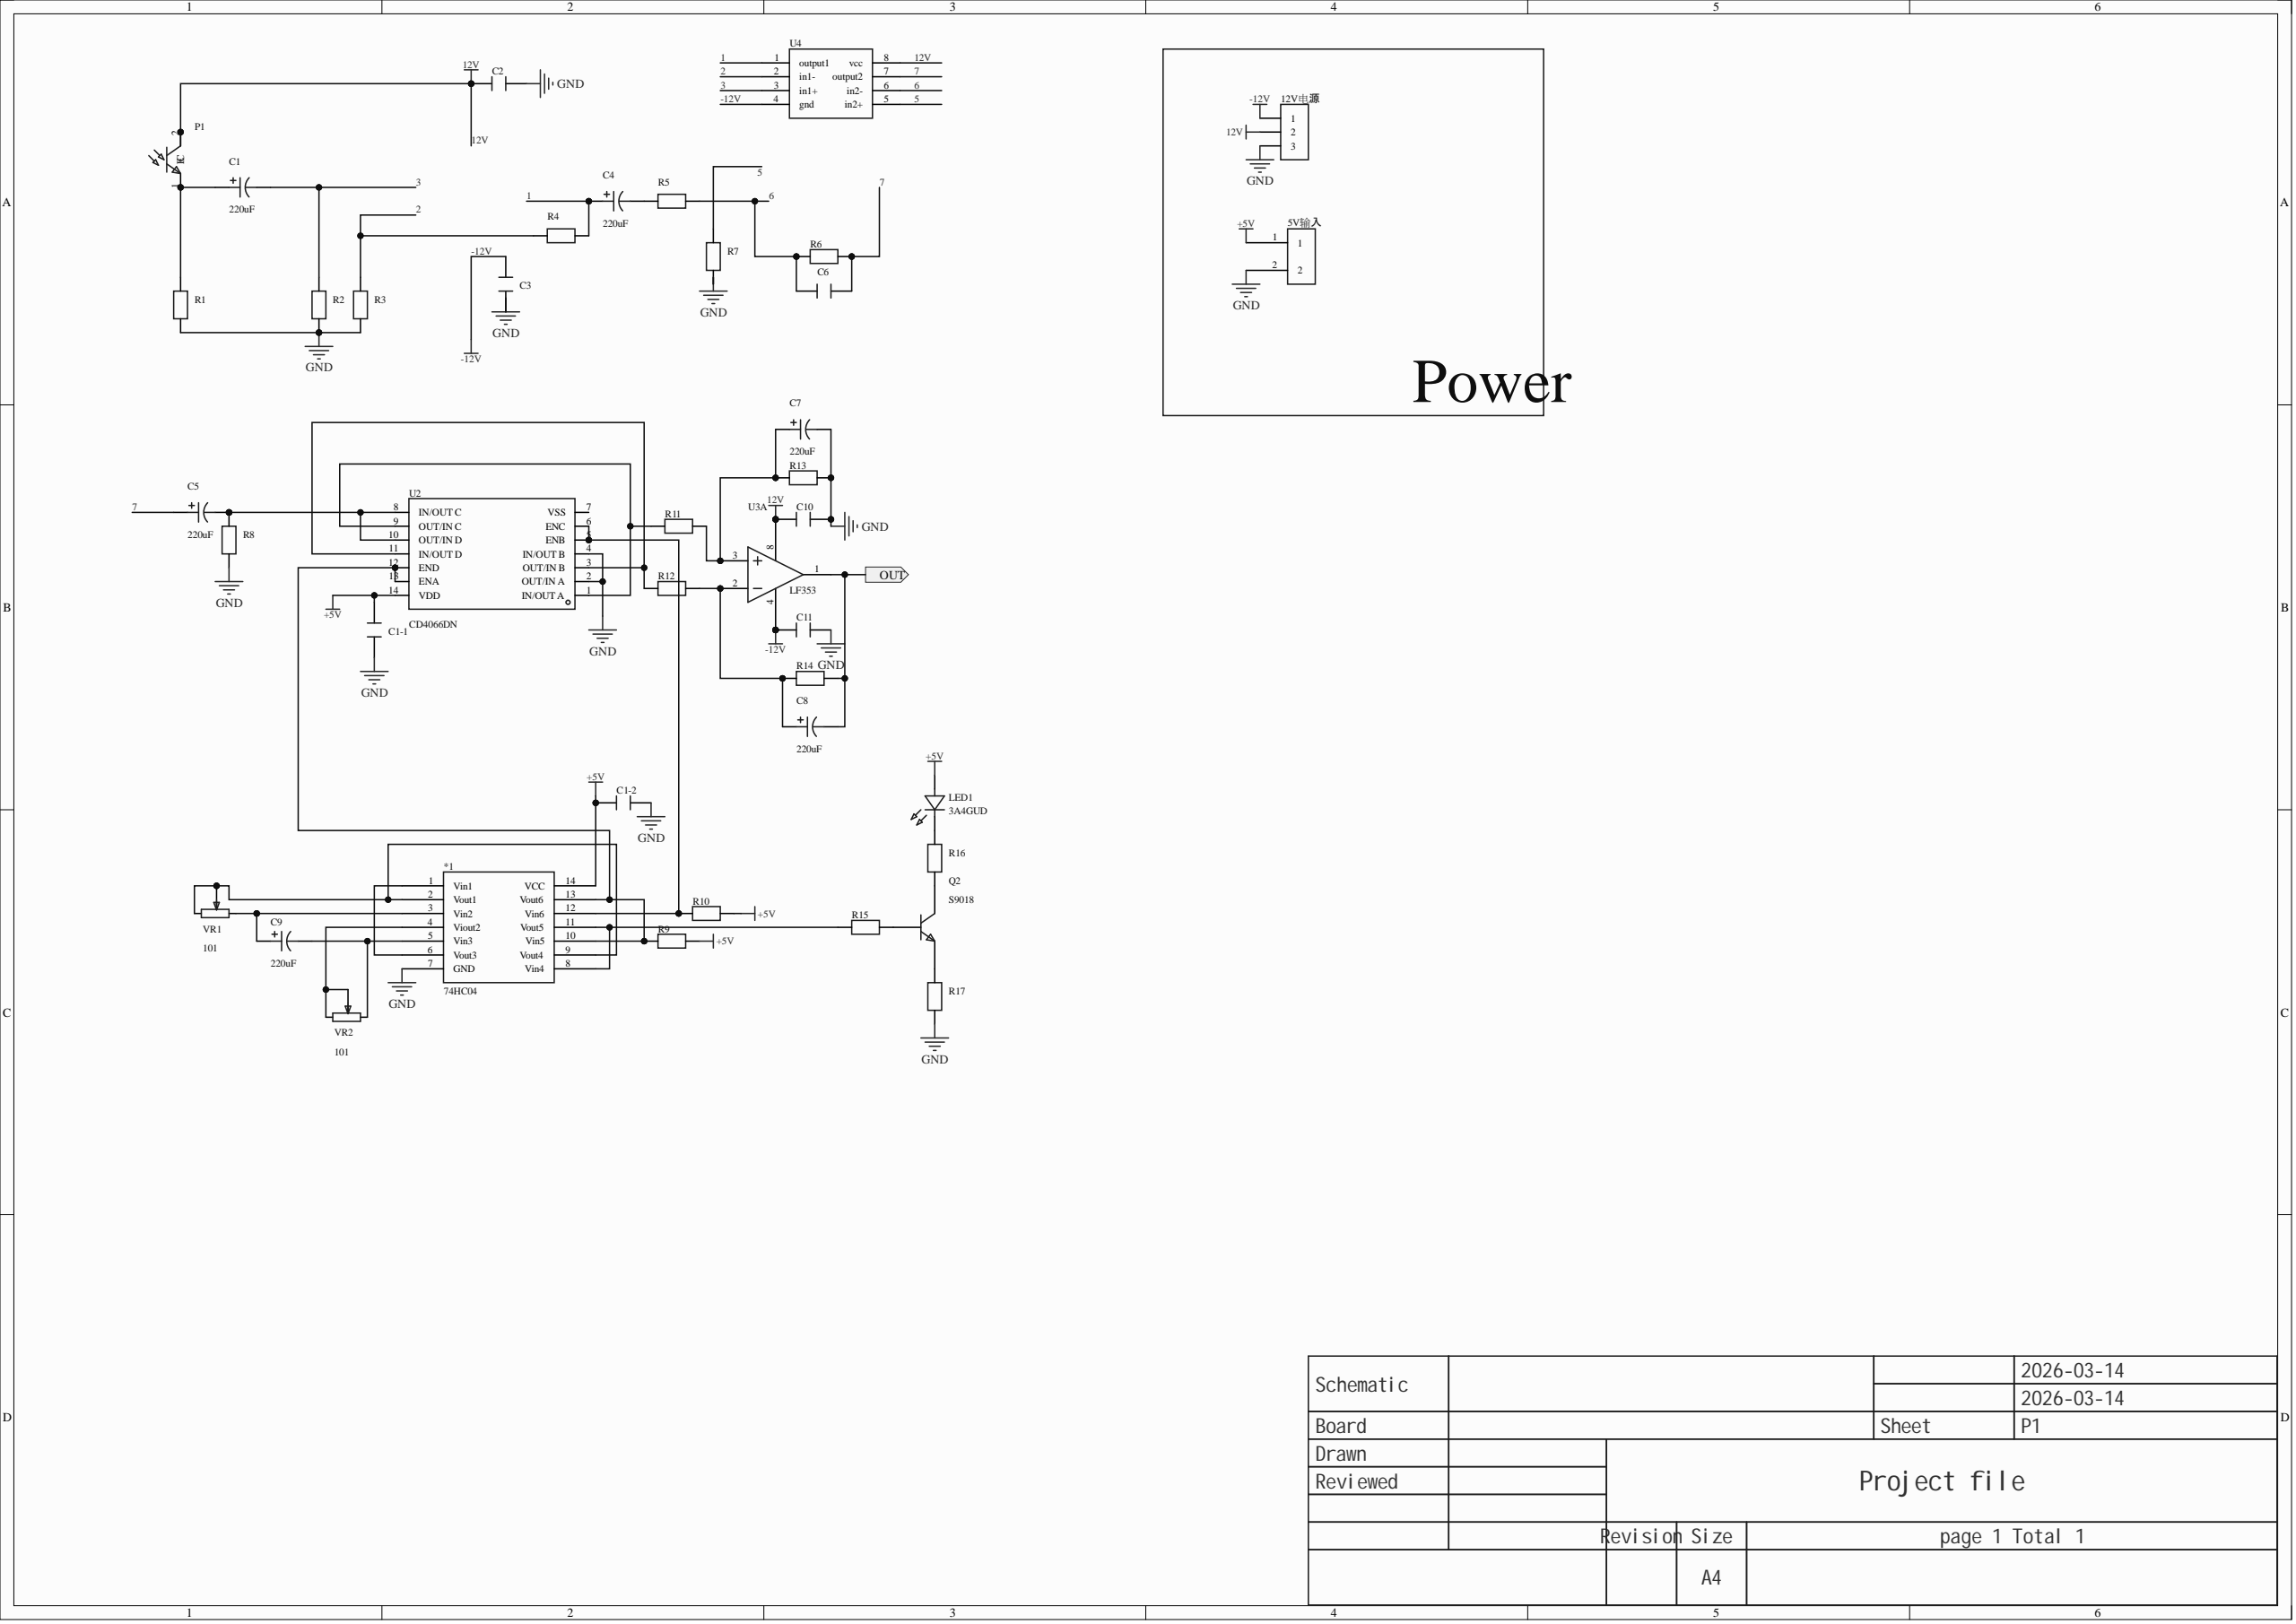Circuit board | Altium Designer | 41 parts | 30 nets
Bill of materials:
Comment,Description,Designator,Footprint,LibRef,Quantity
"74HC04","","*1","DIP14","74HC04","1"
"5V output","","5V输入","2INT","2PIN","1"
"3PIN","","12V电源","3PIN","3PIN","1"
"","","C1-1, C1-2, C2, C3, C6, C10, C11","电容直插","电容直插","7"
"220uF","Capacitance:220uF;Tolerance:±20%;Rated voltage:16V;Ripple current:300mA@100kHz;Equivalent series resistance(ESR):220mO@100kHz;","C1, C4, C5, C7, C8, C9","CAP-TH_BD6.3-P2.50-D0.5-FD","ERG16V220M6X7","6"
"3A4GUD","Lamp holder type:3mm round lamp holder;Illumination color:Emerald green;Forward voltage(Vf):2.8V~3.2V;Forward current:20mA;Wavelength:520nm~525nm;Lens color:Green lens;Color temperature:-;Luminous intensity:8000mcd~12000mcd;Viewing angle:30°;Operating temperature:-40℃~+85℃;","LED1","LED-TH_BD3.5-P2.54-RD-GREEN","3A4GUD","1"
"","","P1","LED_D3.0mm_Horizontal_O1.27mm_Z2.0mm","LED-3MM-红外接收","1"
"S9018","Transistor type:NPN;Collector-emitter breakdown voltage(Vceo):18V;Collector current(Ic):50mA;Power(Pd):400mW;Collector cutoff current(Icbo):100nA;Collector-emitter saturation voltage(VCE(sat)@Ic,Ib):500mV@10mA,1mA;DC current gain(hFE@Ic,Vce):97@1mA,5V;Transition frequency(fT):800MHz;Operating temperature:+150℃@(Tj);","Q2","TO-92-3_L4.9-W3.7-P1.27-L","S9018","1"
"","Through-hole resistor","R1, R2, R3, R4, R5, R6, R7, R8, R9, R10, R11, R12, R13, R14, R15, R16, R17","D45-V(直插)","直插电阻","17"
"CD4066DN","Switch circuit:1:1;Channels:4;On-resistance(Ron):125O;","U2","PDIP-14_L19.3-W6.5-P2.54-LS7.6-BL","CD4066DN","1"
"LF353","","U3","DIP-8","LF353","1"
"","","U4","DIP-8_L9.9-W6.4-P2.54-LS7.6-BL","lf353","1"
"101","","VR1, VR2","3296W","3296","2"
Netlist (Protel format):
[
5V输入
2INT
5V output



]
[
12V电源
3PIN
3PIN



]
[
*1
DIP14
74HC04



]
[
C1
CAP-TH_BD6.3-P2.50-D0.5-FD
220uF



]
[
C1-1
电容直插




]
[
C1-2
电容直插




]
[
C2
电容直插




]
[
C3
电容直插




]
[
C4
CAP-TH_BD6.3-P2.50-D0.5-FD
220uF



]
[
C5
CAP-TH_BD6.3-P2.50-D0.5-FD
220uF



]
[
C6
电容直插




]
[
C7
CAP-TH_BD6.3-P2.50-D0.5-FD
220uF



]
[
C8
CAP-TH_BD6.3-P2.50-D0.5-FD
220uF



]
[
C9
CAP-TH_BD6.3-P2.50-D0.5-FD
220uF



]
[
C10
电容直插




]
[
C11
电容直插




]
[
LED1
LED-TH_BD3.5-P2.54-RD-GREEN
3A4GUD



]
[
P1
LED_D3.0mm_Horizontal_O1.27mm_Z2.0mm




]
[
Q2
TO-92-3_L4.9-W3.7-P1.27-L
S9018



]
[
R1
D45-V(直插)




]
[
R2
D45-V(直插)




]
[
R3
D45-V(直插)




]
[
R4
D45-V(直插)




]
[
R5
D45-V(直插)




]
[
R6
D45-V(直插)




]
[
R7
D45-V(直插)




]
[
R8
D45-V(直插)




]
[
R9
D45-V(直插)




]
[
R10
D45-V(直插)




]
[
R11
D45-V(直插)




]
[
R12
D45-V(直插)




]
[
R13
D45-V(直插)




]
[
R14
D45-V(直插)




]
[
R15
D45-V(直插)




]
[
R16
D45-V(直插)




]
[
R17
D45-V(直插)




]
[
U2
PDIP-14_L19.3-W6.5-P2.54-LS7.6-BL
CD4066DN



]
[
U3
DIP-8
LF353



]
[
U4
DIP-8_L9.9-W6.4-P2.54-LS7.6-BL




]
[
VR1
3296W
101



]
[
VR2
3296W
101



]
(
NetR12_1
R12-1
U2-3
U2-11
)
(
NetR11_1
R11-1
U2-1
U2-9
)
(
NetQ2_3
Q2-3
R16-1
)
(
NetQ2_2
Q2-2
R15-2
)
(
NetQ2_1
Q2-1
R17-2
)
(
NetLED1_1
LED1-1
R16-2
)
(
NetC8_2
C8-2
R14-2
U3-1
)
(
NetC8_1
C8-1
R12-2
R14-1
U3-2
)
(
NetC7_1
C7-1
R11-2
R13-1
U3-3
)
(
NetC5_2
C5-2
R8-1
U2-8
U2-10
)
(
NetC4_2
C4-2
R5-2
)
(
NetC1_1
C1-1
P1-1
R1-1
)
(
Net*1_12
*1-12
R10-1
U2-5
U2-6
)
(
Net*1_10
*1-10
*1-13
R9-1
U2-12
U2-13
)
(
Net*1_8
*1-8
*1-11
R15-1
)
(
Net*1_5
*1-5
C9-2
VR2-3
)
(
Net*1_4
*1-4
VR2-1
VR2-2
)
(
Net*1_3
*1-3
C9-1
VR1-3
)
(
Net*1_2
*1-2
*1-9
VR1-1
VR1-2
)
(
Net*1_1
*1-1
*1-6
)
(
GND
5V输入-2
12V电源-3
*1-7
C1-1-1
C1-2-1
C2-1
C3-1
C7-2
C10-1
C11-1
R1-2
R2-2
R3-2
R7-1
R8-2
R13-2
R17-1
U2-2
U2-4
)
(
-12V
12V电源-1
C3-2
C11-2
U3-4
U4-4
)
(
+5V
5V输入-1
*1-14
C1-1-2
C1-2-2
LED1-2
R9-2
R10-2
U2-14
)
(
12V
12V电源-2
C2-2
C10-2
P1-2
U3-8
U4-8
)
(
7
C5-1
C6-1
R6-2
U4-7
)
(
6
C6-2
R5-1
R6-1
U4-6
)
(
5
R7-2
U4-5
)
(
3
C1-2
R2-1
U4-3
)
(
2
R3-1
R4-2
U4-2
)
(
1
C4-1
R4-1
U4-1
)